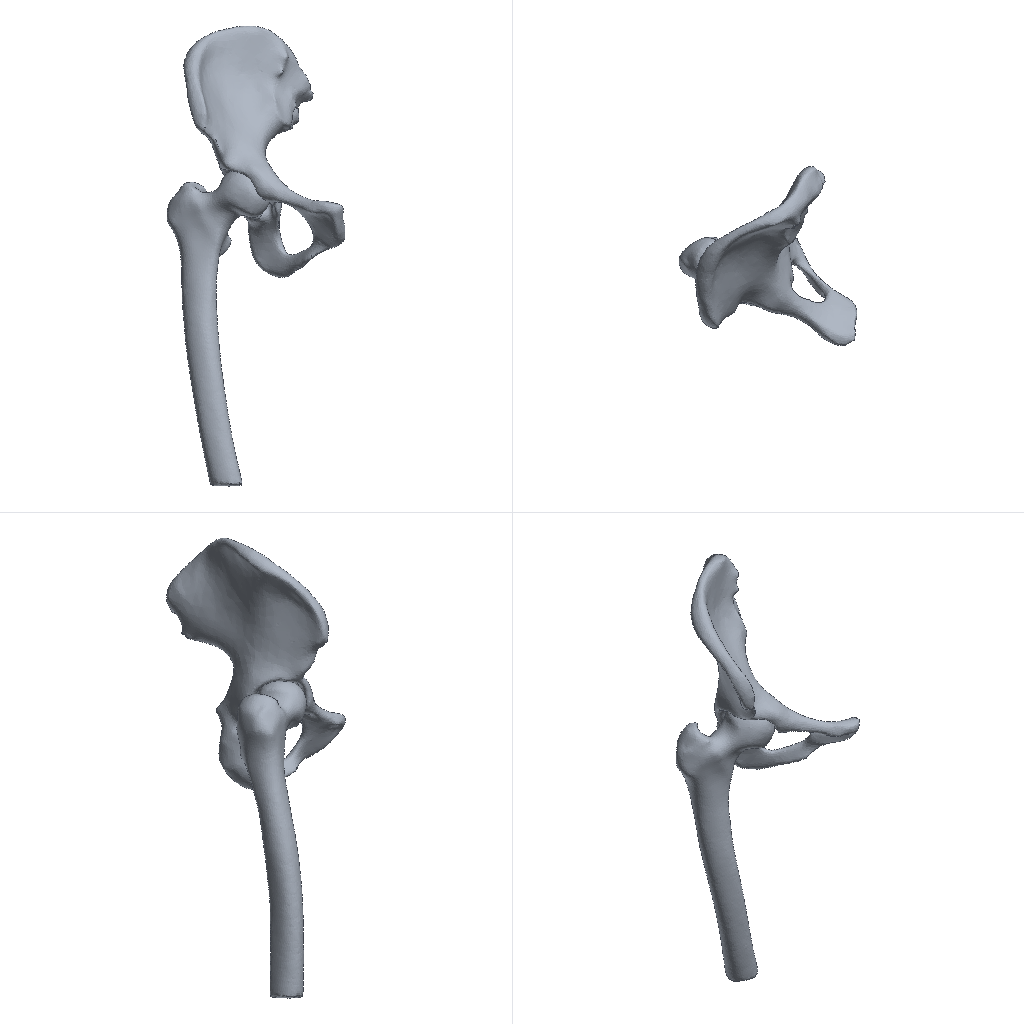Simulation study | abaqus
Set-up summary, first 304 of 512 lines:
category,name,step,type,value,unit,region
solver,abaqus,,Abaqus/CAE 2024
units,unstated,,unstated,E=3.588 density=10 (no match)
analysis,Step-1,,static,time_period=1
mesh,nodes,,,69990
mesh,elements,,,349636
element_type,C3D4,,,349636
material,MAT1,,E,3.588
material,MAT1,,nu,0.3
material,MAT1,,density,10
material,MAT2,,E,3.588
material,MAT2,,nu,0.3
material,MAT2,,density,10
material,MAT3,,E,3.13
material,MAT3,,nu,0.3
material,MAT3,,density,9.163
material,MAT4,,E,25.667
material,MAT4,,nu,0.3
material,MAT4,,density,35.3
material,MAT5,,E,60.925
material,MAT5,,nu,0.3
material,MAT5,,density,61.437
material,MAT6,,E,105.913
material,MAT6,,nu,0.3
material,MAT6,,density,87.574
material,MAT7,,E,159.184
material,MAT7,,nu,0.3
material,MAT7,,density,113.711
material,MAT8,,E,219.822
material,MAT8,,nu,0.3
material,MAT8,,density,139.848
material,MAT9,,E,287.18
material,MAT9,,nu,0.3
material,MAT9,,density,165.985
material,MAT10,,E,360.767
material,MAT10,,nu,0.3
material,MAT10,,density,192.123
material,MAT11,,E,440.194
material,MAT11,,nu,0.3
material,MAT11,,density,218.26
material,MAT12,,E,525.139
material,MAT12,,nu,0.3
material,MAT12,,density,244.397
material,MAT13,,E,615.334
material,MAT13,,nu,0.3
material,MAT13,,density,270.534
material,MAT14,,E,710.549
material,MAT14,,nu,0.3
material,MAT14,,density,296.671
material,MAT15,,E,810.585
material,MAT15,,nu,0.3
material,MAT15,,density,322.808
material,MAT16,,E,915.264
material,MAT16,,nu,0.3
material,MAT16,,density,348.945
material,MAT17,,E,1024.43
material,MAT17,,nu,0.3
material,MAT17,,density,375.083
material,MAT18,,E,1137.94
material,MAT18,,nu,0.3
material,MAT18,,density,401.22
material,MAT19,,E,1255.68
material,MAT19,,nu,0.3
material,MAT19,,density,427.357
material,MAT20,,E,1377.51
material,MAT20,,nu,0.3
material,MAT20,,density,453.494
material,MAT21,,E,1503.35
material,MAT21,,nu,0.3
material,MAT21,,density,479.631
material,MAT22,,E,1633.09
material,MAT22,,nu,0.3
material,MAT22,,density,505.768
material,MAT23,,E,1766.63
material,MAT23,,nu,0.3
material,MAT23,,density,531.905
material,MAT24,,E,1903.91
material,MAT24,,nu,0.3
material,MAT24,,density,558.042
material,MAT25,,E,2044.83
material,MAT25,,nu,0.3
material,MAT25,,density,584.18
material,MAT26,,E,2189.33
material,MAT26,,nu,0.3
material,MAT26,,density,610.317
material,MAT27,,E,2337.34
material,MAT27,,nu,0.3
material,MAT27,,density,636.454
material,MAT28,,E,2488.79
material,MAT28,,nu,0.3
material,MAT28,,density,662.591
material,MAT29,,E,2643.62
material,MAT29,,nu,0.3
material,MAT29,,density,688.728
material,MAT30,,E,2801.78
material,MAT30,,nu,0.3
material,MAT30,,density,714.865
material,MAT31,,E,2963.22
material,MAT31,,nu,0.3
material,MAT31,,density,741.002
material,MAT32,,E,3127.87
material,MAT32,,nu,0.3
material,MAT32,,density,767.139
material,MAT33,,E,3295.7
material,MAT33,,nu,0.3
material,MAT33,,density,793.277
material,MAT34,,E,3466.65
material,MAT34,,nu,0.3
material,MAT34,,density,819.414
material,MAT35,,E,3640.68
material,MAT35,,nu,0.3
material,MAT35,,density,845.551
material,MAT36,,E,3817.76
material,MAT36,,nu,0.3
material,MAT36,,density,871.688
material,MAT37,,E,3997.83
material,MAT37,,nu,0.3
material,MAT37,,density,897.825
material,MAT38,,E,4180.86
material,MAT38,,nu,0.3
material,MAT38,,density,923.962
material,MAT39,,E,4366.81
material,MAT39,,nu,0.3
material,MAT39,,density,950.099
material,MAT40,,E,4555.65
material,MAT40,,nu,0.3
material,MAT40,,density,976.236
material,MAT41,,E,4747.35
material,MAT41,,nu,0.3
material,MAT41,,density,1002.37
material,MAT42,,E,4941.86
material,MAT42,,nu,0.3
material,MAT42,,density,1028.51
material,MAT43,,E,5139.16
material,MAT43,,nu,0.3
material,MAT43,,density,1054.65
material,MAT44,,E,5339.22
material,MAT44,,nu,0.3
material,MAT44,,density,1080.78
material,MAT45,,E,5542.01
material,MAT45,,nu,0.3
material,MAT45,,density,1106.92
material,MAT46,,E,5747.5
material,MAT46,,nu,0.3
material,MAT46,,density,1133.06
material,MAT47,,E,5955.66
material,MAT47,,nu,0.3
material,MAT47,,density,1159.2
material,MAT48,,E,6166.46
material,MAT48,,nu,0.3
material,MAT48,,density,1185.33
material,MAT49,,E,6379.89
material,MAT49,,nu,0.3
material,MAT49,,density,1211.47
material,MAT50,,E,6595.9
material,MAT50,,nu,0.3
material,MAT50,,density,1237.61
material,MAT51,,E,6814.49
material,MAT51,,nu,0.3
material,MAT51,,density,1263.74
material,MAT52,,E,7035.63
material,MAT52,,nu,0.3
material,MAT52,,density,1289.88
material,MAT53,,E,7259.29
material,MAT53,,nu,0.3
material,MAT53,,density,1316.02
material,MAT54,,E,7485.45
material,MAT54,,nu,0.3
material,MAT54,,density,1342.16
material,MAT55,,E,7714.09
material,MAT55,,nu,0.3
material,MAT55,,density,1368.29
material,MAT56,,E,7945.18
material,MAT56,,nu,0.3
material,MAT56,,density,1394.43
material,MAT57,,E,8178.72
material,MAT57,,nu,0.3
material,MAT57,,density,1420.57
material,MAT58,,E,8414.68
material,MAT58,,nu,0.3
material,MAT58,,density,1446.7
material,MAT59,,E,8653.03
material,MAT59,,nu,0.3
material,MAT59,,density,1472.84
material,MAT60,,E,8893.77
material,MAT60,,nu,0.3
material,MAT60,,density,1498.98
material,MAT61,,E,9136.87
material,MAT61,,nu,0.3
material,MAT61,,density,1525.12
material,MAT62,,E,9382.31
material,MAT62,,nu,0.3
material,MAT62,,density,1551.25
material,MAT63,,E,9630.08
material,MAT63,,nu,0.3
material,MAT63,,density,1577.39
material,MAT64,,E,9880.16
material,MAT64,,nu,0.3
material,MAT64,,density,1603.53
material,MAT65,,E,10132.5
material,MAT65,,nu,0.3
material,MAT65,,density,1629.66
material,MAT66,,E,10387.2
material,MAT66,,nu,0.3
material,MAT66,,density,1655.8
material,MAT67,,E,10644.1
material,MAT67,,nu,0.3
material,MAT67,,density,1681.94
material,MAT68,,E,10903.3
material,MAT68,,nu,0.3
material,MAT68,,density,1708.08
material,MAT69,,E,11164.6
material,MAT69,,nu,0.3
material,MAT69,,density,1734.21
material,MAT70,,E,11428.2
material,MAT70,,nu,0.3
material,MAT70,,density,1760.35
material,MAT71,,E,11694
material,MAT71,,nu,0.3
material,MAT71,,density,1786.49
material,MAT72,,E,11962
material,MAT72,,nu,0.3
material,MAT72,,density,1812.62
material,MAT73,,E,12232.2
material,MAT73,,nu,0.3
material,MAT73,,density,1838.76
material,MAT74,,E,12504.5
material,MAT74,,nu,0.3
material,MAT74,,density,1864.9
material,MAT75,,E,12779
material,MAT75,,nu,0.3
material,MAT75,,density,1891.04
material,MAT76,,E,13055.6
material,MAT76,,nu,0.3
material,MAT76,,density,1917.17
material,MAT77,,E,13334.3
material,MAT77,,nu,0.3
material,MAT77,,density,1943.31
material,MAT78,,E,13615.1
material,MAT78,,nu,0.3
material,MAT78,,density,1969.45
material,MAT79,,E,13898.1
material,MAT79,,nu,0.3
material,MAT79,,density,1995.58
material,MAT80,,E,14183.1
material,MAT80,,nu,0.3
material,MAT80,,density,2021.72
material,MAT81,,E,14470.1
material,MAT81,,nu,0.3
material,MAT81,,density,2047.86
material,MAT82,,E,14759.3
material,MAT82,,nu,0.3
material,MAT82,,density,2074
material,MAT83,,E,15050.5
material,MAT83,,nu,0.3
material,MAT83,,density,2100.13
material,MAT84,,E,15343.7
material,MAT84,,nu,0.3
material,MAT84,,density,2126.27
material,MAT85,,E,15638.9
material,MAT85,,nu,0.3
material,MAT85,,density,2152.41
material,MAT86,,E,15936.2
material,MAT86,,nu,0.3
material,MAT86,,density,2178.54
material,MAT87,,E,16235.5
material,MAT87,,nu,0.3
material,MAT87,,density,2204.68
material,MAT88,,E,16536.7
material,MAT88,,nu,0.3
material,MAT88,,density,2230.82
material,MAT89,,E,16840
material,MAT89,,nu,0.3
material,MAT89,,density,2256.96
material,MAT90,,E,17145.2
material,MAT90,,nu,0.3
material,MAT90,,density,2283.09
material,MAT91,,E,17452.3
material,MAT91,,nu,0.3
material,MAT91,,density,2309.23
material,MAT92,,E,17761.5
material,MAT92,,nu,0.3
material,MAT92,,density,2335.37
material,MAT93,,E,18072.5
material,MAT93,,nu,0.3
material,MAT93,,density,2361.5
material,MAT94,,E,18385.6
material,MAT94,,nu,0.3
material,MAT94,,density,2387.64
material,MAT95,,E,18700.5
material,MAT95,,nu,0.3
material,MAT95,,density,2413.78
material,MAT96,,E,19017.3
material,MAT96,,nu,0.3
material,MAT96,,density,2439.92
material,MAT97,,E,19336.1
material,MAT97,,nu,0.3
material,MAT97,,density,2466.05
material,MAT98,,E,19656.7
material,MAT98,,nu,0.3
material,MAT98,,density,2492.19
material,MAT99,,E,19979.3
material,MAT99,,nu,0.3
material,MAT99,,density,2518.33
Abaqus input file, long lists of numbers shortened:
*Heading
** Job name: deck Model name: Model-1
** Generated by: Abaqus/CAE 2024
*Preprint, echo=NO, model=NO, history=NO, contact=NO
**
** PARTS
**
*Part, name=PART-1
*Node
      1,   130.489,   178.725,  -456.04
      2,     128.38,   180.805,  -455.985
** (42545 more lines like these left out)
*Element, type=C3D4
     1, 15021, 15022, 15023, 15024
     2, 15052, 15056, 15061, 15060
** (209817 more lines like these left out)
*Elset, elset=SET1, generate
    1,  5544,     1
*Elset, elset=SET2, generate
  5545,  11304,      1
*Elset, elset=SET3, generate
 11305,  17139,      1
*Elset, elset=SET4, generate
 17140,  21919,      1
*Elset, elset=SET5, generate
 21920,  26644,      1
*Elset, elset=SET6, generate
 26645,  31174,      1
*Elset, elset=SET7, generate
 31175,  35879,      1
*Elset, elset=SET8, generate
 35880,  40947,      1
*Elset, elset=SET9, generate
 40948,  45595,      1
*Elset, elset=SET10, generate
 45596,  50282,      1
*Elset, elset=SET11, generate
 50283,  54802,      1
*Elset, elset=SET12, generate
 54803,  60110,      1
*Elset, elset=SET13, generate
 60111,  64878,      1
*Elset, elset=SET14, generate
 64879,  69715,      1
*Elset, elset=SET15, generate
 69716,  75415,      1
*Elset, elset=SET16, generate
 75416,  80360,      1
*Elset, elset=SET17, generate
 80361,  85668,      1
*Elset, elset=SET18, generate
 85669,  88539,      1
*Elset, elset=SET19, generate
 88540,  92539,      1
*Elset, elset=SET20, generate
 92540,  97409,      1
*Elset, elset=SET21, generate
  97410,  101380,       1
*Elset, elset=SET22, generate
 101381,  104554,       1
*Elset, elset=SET23, generate
 104555,  108745,       1
*Elset, elset=SET24, generate
 108746,  111019,       1
*Elset, elset=SET25, generate
 111020,  114768,       1
*Elset, elset=SET26, generate
 114769,  118305,       1
*Elset, elset=SET27, generate
 118306,  118406,       1
*Elset, elset=SET28, generate
 118407,  120989,       1
*Elset, elset=SET29, generate
 120990,  124573,       1
*Elset, elset=SET30, generate
 124574,  126890,       1
*Elset, elset=SET31, generate
 126891,  130256,       1
*Elset, elset=SET32, generate
 130257,  133204,       1
*Elset, elset=SET33, generate
 133205,  137274,       1
*Elset, elset=SET34, generate
 137275,  139342,       1
*Elset, elset=SET35, generate
 139343,  143097,       1
*Elset, elset=SET36, generate
 143098,  146468,       1
*Elset, elset=SET37, generate
 146469,  150080,       1
*Elset, elset=SET38, generate
 150081,  151210,       1
*Elset, elset=SET39, generate
 151211,  153627,       1
*Elset, elset=SET40, generate
 153628,  155034,       1
*Elset, elset=SET41, generate
 155035,  156868,       1
*Elset, elset=SET42, generate
 156869,  159876,       1
*Elset, elset=SET43, generate
 159877,  162662,       1
*Elset, elset=SET44, generate
 162663,  165367,       1
*Elset, elset=SET45, generate
 165368,  167319,       1
*Elset, elset=SET46, generate
 167320,  167831,       1
*Elset, elset=SET47, generate
 167832,  170587,       1
*Elset, elset=SET48, generate
 170588,  171822,       1
*Elset, elset=SET49, generate
 171823,  174996,       1
*Elset, elset=SET50, generate
 174997,  175669,       1
*Elset, elset=SET51, generate
 175670,  178846,       1
*Elset, elset=SET52, generate
 178847,  179828,       1
*Elset, elset=SET53, generate
 179829,  181183,       1
*Elset, elset=SET54, generate
 181184,  182916,       1
*Elset, elset=SET55, generate
 182917,  183902,       1
*Elset, elset=SET56, generate
 183903,  184076,       1
*Elset, elset=SET57, generate
 184077,  184573,       1
*Elset, elset=SET58, generate
 184574,  186976,       1
*Elset, elset=SET59, generate
 186977,  187814,       1
*Elset, elset=SET60, generate
 187815,  189490,       1
*Elset, elset=SET61, generate
 189491,  189706,       1
*Elset, elset=SET62, generate
 189707,  191900,       1
*Elset, elset=SET63, generate
 191901,  193163,       1
*Elset, elset=SET64, generate
 193164,  195027,       1
*Elset, elset=SET65, generate
 195028,  195725,       1
*Elset, elset=SET66, generate
 195726,  196332,       1
*Elset, elset=SET67, generate
 196333,  197612,       1
*Elset, elset=SET68, generate
 197613,  199159,       1
*Elset, elset=SET69, generate
 199160,  200649,       1
*Elset, elset=SET70, generate
 200650,  201547,       1
*Elset, elset=SET71, generate
 201548,  202707,       1
*Elset, elset=SET72, generate
 202708,  203378,       1
*Elset, elset=SET73, generate
 203379,  203387,       1
*Elset, elset=SET74, generate
 203388,  203647,       1
*Elset, elset=SET75, generate
 203648,  205094,       1
*Elset, elset=SET76, generate
 205095,  205226,       1
*Elset, elset=SET77, generate
 205227,  205780,       1
*Elset, elset=SET78, generate
 205781,  205844,       1
*Elset, elset=SET79, generate
 205845,  206302,       1
*Elset, elset=SET80, generate
 206303,  206457,       1
*Elset, elset=SET81, generate
 206458,  206530,       1
*Elset, elset=SET82, generate
 206531,  206832,       1
*Elset, elset=SET83, generate
 206833,  206849,       1
*Elset, elset=SET84, generate
 206850,  207592,       1
*Elset, elset=SET85, generate
 207593,  207931,       1
*Elset, elset=SET86, generate
 207932,  208213,       1
*Elset, elset=SET87, generate
 208214,  208584,       1
*Elset, elset=SET88, generate
 208585,  208647,       1
*Elset, elset=SET89, generate
 208648,  208986,       1
*Elset, elset=SET90, generate
 208987,  208994,       1
*Elset, elset=SET91, generate
 208995,  209235,       1
*Elset, elset=SET92, generate
 209236,  209268,       1
*Elset, elset=SET93, generate
 209269,  209473,       1
*Elset, elset=SET94, generate
 209474,  209665,       1
*Elset, elset=SET95, generate
 209666,  209783,       1
*Elset, elset=SET96, generate
 209784,  209799,       1
*Elset, elset=SET97, generate
 209800,  209807,       1
*Elset, elset=SET98, generate
 209808,  209811,       1
*Elset, elset=SET99, generate
 209812,  209818,       1
*Elset, elset=SET100
 209819,
** Section: Section-1-SET1
*Solid Section, elset=SET1, material=MAT21
,
** Section: Section-2-SET2
*Solid Section, elset=SET2, material=MAT65
,
** Section: Section-3-SET3
*Solid Section, elset=SET3, material=MAT36
,
** Section: Section-4-SET4
*Solid Section, elset=SET4, material=MAT31
,
** Section: Section-5-SET5
*Solid Section, elset=SET5, material=MAT32
,
** Section: Section-6-SET6
*Solid Section, elset=SET6, material=MAT20
,
** Section: Section-7-SET7
*Solid Section, elset=SET7, material=MAT22
,
** Section: Section-8-SET8
*Solid Section, elset=SET8, material=MAT33
,
** Section: Section-9-SET9
*Solid Section, elset=SET9, material=MAT27
,
** Section: Section-10-SET10
*Solid Section, elset=SET10, material=MAT34
,
** Section: Section-11-SET11
*Solid Section, elset=SET11, material=MAT11
,
** Section: Section-12-SET12
*Solid Section, elset=SET12, material=MAT10
,
** Section: Section-13-SET13
*Solid Section, elset=SET13, material=MAT96
,
** Section: Section-14-SET14
*Solid Section, elset=SET14, material=MAT14
,
** Section: Section-15-SET15
*Solid Section, elset=SET15, material=MAT83
,
** Section: Section-16-SET16
*Solid Section, elset=SET16, material=MAT8
,
** Section: Section-17-SET17
*Solid Section, elset=SET17, material=MAT12
,
** Section: Section-18-SET18
*Solid Section, elset=SET18, material=MAT9
,
** Section: Section-19-SET19
*Solid Section, elset=SET19, material=MAT17
,
** Section: Section-20-SET20
*Solid Section, elset=SET20, material=MAT28
,
** Section: Section-21-SET21
*Solid Section, elset=SET21, material=MAT40
,
** Section: Section-22-SET22
*Solid Section, elset=SET22, material=MAT35
,
** Section: Section-23-SET23
*Solid Section, elset=SET23, material=MAT29
,
** Section: Section-24-SET24
*Solid Section, elset=SET24, material=MAT26
,
** Section: Section-25-SET25
*Solid Section, elset=SET25, material=MAT25
,
** Section: Section-26-SET26
*Solid Section, elset=SET26, material=MAT23
,
** Section: Section-27-SET27
*Solid Section, elset=SET27, material=MAT7
,
** Section: Section-28-SET28
*Solid Section, elset=SET28, material=MAT41
,
** Section: Section-29-SET29
*Solid Section, elset=SET29, material=MAT19
,
** Section: Section-30-SET30
*Solid Section, elset=SET30, material=MAT42
,
** Section: Section-31-SET31
*Solid Section, elset=SET31, material=MAT13
,
** Section: Section-32-SET32
*Solid Section, elset=SET32, material=MAT16
,
** Section: Section-33-SET33
*Solid Section, elset=SET33, material=MAT30
,
** Section: Section-34-SET34
*Solid Section, elset=SET34, material=MAT37
,
** Section: Section-35-SET35
*Solid Section, elset=SET35, material=MAT46
,
** Section: Section-36-SET36
*Solid Section, elset=SET36, material=MAT15
,
** Section: Section-37-SET37
*Solid Section, elset=SET37, material=MAT91
,
** Section: Section-38-SET38
*Solid Section, elset=SET38, material=MAT6
,
** Section: Section-39-SET39
*Solid Section, elset=SET39, material=MAT4
,
** Section: Section-40-SET40
*Solid Section, elset=SET40, material=MAT2
,
** Section: Section-41-SET41
*Solid Section, elset=SET41, material=MAT3
,
** Section: Section-42-SET42
*Solid Section, elset=SET42, material=MAT5
,
** Section: Section-43-SET43
*Solid Section, elset=SET43, material=MAT39
,
** Section: Section-44-SET44
*Solid Section, elset=SET44, material=MAT90
,
** Section: Section-45-SET45
*Solid Section, elset=SET45, material=MAT38
,
** Section: Section-46-SET46
*Solid Section, elset=SET46, material=MAT80
,
** Section: Section-47-SET47
*Solid Section, elset=SET47, material=MAT52
,
** Section: Section-48-SET48
*Solid Section, elset=SET48, material=MAT86
,
** Section: Section-49-SET49
*Solid Section, elset=SET49, material=MAT24
,
** Section: Section-50-SET50
*Solid Section, elset=SET50, material=MAT43
,
** Section: Section-51-SET51
*Solid Section, elset=SET51, material=MAT76
,
** Section: Section-52-SET52
*Solid Section, elset=SET52, material=MAT95
,
** Section: Section-53-SET53
*Solid Section, elset=SET53, material=MAT93
,
** Section: Section-54-SET54
*Solid Section, elset=SET54, material=MAT89
,
** Section: Section-55-SET55
*Solid Section, elset=SET55, material=MAT45
,
** Section: Section-56-SET56
*Solid Section, elset=SET56, material=MAT44
,
** Section: Section-57-SET57
*Solid Section, elset=SET57, material=MAT18
,
** Section: Section-58-SET58
*Solid Section, elset=SET58, material=MAT54
,
** Section: Section-59-SET59
*Solid Section, elset=SET59, material=MAT77
,
** Section: Section-60-SET60
*Solid Section, elset=SET60, material=MAT71
,
** Section: Section-61-SET61
*Solid Section, elset=SET61, material=MAT55
,
** Section: Section-62-SET62
*Solid Section, elset=SET62, material=MAT73
,
** Section: Section-63-SET63
*Solid Section, elset=SET63, material=MAT47
,
** Section: Section-64-SET64
*Solid Section, elset=SET64, material=MAT67
,
** Section: Section-65-SET65
*Solid Section, elset=SET65, material=MAT81
,
** Section: Section-66-SET66
*Solid Section, elset=SET66, material=MAT59
,
** Section: Section-67-SET67
*Solid Section, elset=SET67, material=MAT78
,
** Section: Section-68-SET68
*Solid Section, elset=SET68, material=MAT49
,
** Section: Section-69-SET69
*Solid Section, elset=SET69, material=MAT51
,
** Section: Section-70-SET70
*Solid Section, elset=SET70, material=MAT87
,
** Section: Section-71-SET71
*Solid Section, elset=SET71, material=MAT74
,
** Section: Section-72-SET72
*Solid Section, elset=SET72, material=MAT88
,
** Section: Section-73-SET73
*Solid Section, elset=SET73, material=MAT62
,
** Section: Section-74-SET74
*Solid Section, elset=SET74, material=MAT58
,
** Section: Section-75-SET75
*Solid Section, elset=SET75, material=MAT53
,
** Section: Section-76-SET76
*Solid Section, elset=SET76, material=MAT82
,
** Section: Section-77-SET77
*Solid Section, elset=SET77, material=MAT92
,
** Section: Section-78-SET78
*Solid Section, elset=SET78, material=MAT57
,
** Section: Section-79-SET79
*Solid Section, elset=SET79, material=MAT68
,
** Section: Section-80-SET80
*Solid Section, elset=SET80, material=MAT97
,
** Section: Section-81-SET81
*Solid Section, elset=SET81, material=MAT60
,
** Section: Section-82-SET82
*Solid Section, elset=SET82, material=MAT1
,
** Section: Section-83-SET83
*Solid Section, elset=SET83, material=MAT61
,
** Section: Section-84-SET84
*Solid Section, elset=SET84, material=MAT50
,
** Section: Section-85-SET85
*Solid Section, elset=SET85, material=MAT66
,
** Section: Section-86-SET86
*Solid Section, elset=SET86, material=MAT84
,
** Section: Section-87-SET87
*Solid Section, elset=SET87, material=MAT63
,
** Section: Section-88-SET88
*Solid Section, elset=SET88, material=MAT85
,
** Section: Section-89-SET89
*Solid Section, elset=SET89, material=MAT64
,
** Section: Section-90-SET90
*Solid Section, elset=SET90, material=MAT94
,
** Section: Section-91-SET91
*Solid Section, elset=SET91, material=MAT56
,
** Section: Section-92-SET92
*Solid Section, elset=SET92, material=MAT72
,
** Section: Section-93-SET93
*Solid Section, elset=SET93, material=MAT75
,
** Section: Section-94-SET94
*Solid Section, elset=SET94, material=MAT48
,
** Section: Section-95-SET95
*Solid Section, elset=SET95, material=MAT79
,
** Section: Section-96-SET96
*Solid Section, elset=SET96, material=MAT69
,
** Section: Section-97-SET97
*Solid Section, elset=SET97, material=MAT70
,
** Section: Section-98-SET98
*Solid Section, elset=SET98, material=MAT99
,
** Section: Section-99-SET99
*Solid Section, elset=SET99, material=MAT98
,
** Section: Section-100-SET100
*Solid Section, elset=SET100, material=MAT100
,
*End Part
**
*Part, name=PART-2
*Node
      1,   84.384,   152.255,  -622.89
      2,    85.776,   150.316,  -622.89
** (27441 more lines like these left out)
*Element, type=C3D4
     1,  8146,  8147,  8148,  8149
     2,  8238,  8239,  8240,  8241
** (139815 more lines like these left out)
*Elset, elset=SET1, generate
    1,  2335,     1
*Elset, elset=SET2, generate
 2336,  3097,     1
*Elset, elset=SET3, generate
 3098,  4149,     1
*Elset, elset=SET4, generate
 4150,  5553,     1
*Elset, elset=SET5, generate
 5554,  6887,     1
*Elset, elset=SET6, generate
 6888,  9154,     1
*Elset, elset=SET7, generate
  9155,  11513,      1
*Elset, elset=SET8, generate
 11514,  12802,      1
*Elset, elset=SET9, generate
 12803,  14643,      1
*Elset, elset=SET10, generate
 14644,  15767,      1
*Elset, elset=SET11, generate
 15768,  18886,      1
*Elset, elset=SET12, generate
 18887,  22084,      1
*Elset, elset=SET13, generate
 22085,  22681,      1
*Elset, elset=SET14, generate
 22682,  25288,      1
*Elset, elset=SET15, generate
 25289,  26507,      1
*Elset, elset=SET16, generate
 26508,  29349,      1
*Elset, elset=SET17, generate
 29350,  32184,      1
*Elset, elset=SET18, generate
 32185,  35205,      1
*Elset, elset=SET19, generate
 35206,  37703,      1
*Elset, elset=SET20, generate
 37704,  39334,      1
*Elset, elset=SET21, generate
 39335,  40183,      1
*Elset, elset=SET22, generate
 40184,  41305,      1
*Elset, elset=SET23, generate
 41306,  42847,      1
*Elset, elset=SET24, generate
 42848,  44901,      1
*Elset, elset=SET25, generate
 44902,  47087,      1
*Elset, elset=SET26, generate
 47088,  49240,      1
*Elset, elset=SET27, generate
 49241,  51990,      1
*Elset, elset=SET28, generate
 51991,  52916,      1
*Elset, elset=SET29, generate
 52917,  55309,      1
*Elset, elset=SET30, generate
 55310,  56192,      1
*Elset, elset=SET31, generate
 56193,  58885,      1
*Elset, elset=SET32, generate
 58886,  61412,      1
*Elset, elset=SET33, generate
 61413,  62931,      1
*Elset, elset=SET34, generate
 62932,  64000,      1
*Elset, elset=SET35, generate
 64001,  64801,      1
*Elset, elset=SET36, generate
 64802,  67370,      1
*Elset, elset=SET37, generate
 67371,  70024,      1
*Elset, elset=SET38, generate
 70025,  72673,      1
*Elset, elset=SET39, generate
 72674,  74527,      1
*Elset, elset=SET40, generate
 74528,  74897,      1
*Elset, elset=SET41, generate
 74898,  75883,      1
*Elset, elset=SET42, generate
 75884,  78340,      1
*Elset, elset=SET43, generate
 78341,  79304,      1
*Elset, elset=SET44, generate
 79305,  81908,      1
*Elset, elset=SET45, generate
 81909,  82930,      1
*Elset, elset=SET46, generate
 82931,  83998,      1
*Elset, elset=SET47, generate
 83999,  84855,      1
*Elset, elset=SET48, generate
 84856,  86755,      1
*Elset, elset=SET49, generate
 86756,  89023,      1
*Elset, elset=SET50, generate
 89024,  89864,      1
*Elset, elset=SET51, generate
 89865,  90735,      1
*Elset, elset=SET52, generate
 90736,  91954,      1
*Elset, elset=SET53, generate
 91955,  94110,      1
*Elset, elset=SET54, generate
 94111,  96693,      1
*Elset, elset=SET55, generate
 96694,  97444,      1
*Elset, elset=SET56, generate
 97445,  98232,      1
*Elset, elset=SET57, generate
  98233,  100679,       1
*Elset, elset=SET58, generate
 100680,  101512,       1
*Elset, elset=SET59, generate
 101513,  102438,       1
*Elset, elset=SET60, generate
 102439,  103233,       1
*Elset, elset=SET61, generate
 103234,  104059,       1
*Elset, elset=SET62, generate
 104060,  104899,       1
*Elset, elset=SET63, generate
 104900,  105728,       1
*Elset, elset=SET64, generate
 105729,  106519,       1
*Elset, elset=SET65, generate
 106520,  107514,       1
*Elset, elset=SET66, generate
 107515,  108291,       1
*Elset, elset=SET67, generate
 108292,  109246,       1
*Elset, elset=SET68, generate
 109247,  110107,       1
*Elset, elset=SET69, generate
 110108,  110992,       1
*Elset, elset=SET70, generate
 110993,  113025,       1
*Elset, elset=SET71, generate
 113026,  113898,       1
*Elset, elset=SET72, generate
 113899,  116284,       1
*Elset, elset=SET73, generate
 116285,  117031,       1
*Elset, elset=SET74, generate
 117032,  117782,       1
*Elset, elset=SET75, generate
 117783,  118617,       1
*Elset, elset=SET76, generate
 118618,  119815,       1
*Elset, elset=SET77, generate
 119816,  122531,       1
*Elset, elset=SET78, generate
 122532,  123263,       1
*Elset, elset=SET79, generate
 123264,  124071,       1
*Elset, elset=SET80, generate
 124072,  124307,       1
*Elset, elset=SET81, generate
 124308,  125023,       1
*Elset, elset=SET82, generate
 125024,  125089,       1
*Elset, elset=SET83, generate
 125090,  125884,       1
*Elset, elset=SET84, generate
 125885,  126748,       1
*Elset, elset=SET85, generate
 126749,  127475,       1
*Elset, elset=SET86, generate
 127476,  128877,       1
*Elset, elset=SET87, generate
 128878,  129637,       1
*Elset, elset=SET88, generate
 129638,  131173,       1
*Elset, elset=SET89, generate
 131174,  131920,       1
*Elset, elset=SET90, generate
 131921,  133702,       1
*Elset, elset=SET91, generate
 133703,  134533,       1
*Elset, elset=SET92, generate
 134534,  135387,       1
*Elset, elset=SET93, generate
 135388,  136238,       1
*Elset, elset=SET94, generate
 136239,  137053,       1
*Elset, elset=SET95, generate
 137054,  138015,       1
*Elset, elset=SET96, generate
 138016,  138823,       1
*Elset, elset=SET97, generate
 138824,  139639,       1
*Elset, elset=SET98, generate
 139640,  139707,       1
*Elset, elset=SET99, generate
 139708,  139797,       1
*Elset, elset=SET100, generate
 139798,  139817,       1
** Section: Section-1-SET1
*Solid Section, elset=SET1, material=MAT21
,
** Section: Section-2-SET2
*Solid Section, elset=SET2, material=MAT65
,
** Section: Section-3-SET3
*Solid Section, elset=SET3, material=MAT36
,
** Section: Section-4-SET4
*Solid Section, elset=SET4, material=MAT31
,
** Section: Section-5-SET5
*Solid Section, elset=SET5, material=MAT32
,
** Section: Section-6-SET6
*Solid Section, elset=SET6, material=MAT20
,
** Section: Section-7-SET7
*Solid Section, elset=SET7, material=MAT22
,
** Section: Section-8-SET8
*Solid Section, elset=SET8, material=MAT33
,
** Section: Section-9-SET9
*Solid Section, elset=SET9, material=MAT27
,
** Section: Section-10-SET10
*Solid Section, elset=SET10, material=MAT34
,
** Section: Section-11-SET11
*Solid Section, elset=SET11, material=MAT11
,
** Section: Section-12-SET12
*Solid Section, elset=SET12, material=MAT10
,
** Section: Section-13-SET13
*Solid Section, elset=SET13, material=MAT96
,
** Section: Section-14-SET14
*Solid Section, elset=SET14, material=MAT14
,
** Section: Section-15-SET15
*Solid Section, elset=SET15, material=MAT83
,
** Section: Section-16-SET16
*Solid Section, elset=SET16, material=MAT8
,
** Section: Section-17-SET17
*Solid Section, elset=SET17, material=MAT12
,
** Section: Section-18-SET18
*Solid Section, elset=SET18, material=MAT9
,
** Section: Section-19-SET19
*Solid Section, elset=SET19, material=MAT17
,
** Section: Section-20-SET20
*Solid Section, elset=SET20, material=MAT28
,
** Section: Section-21-SET21
*Solid Section, elset=SET21, material=MAT40
,
** Section: Section-22-SET22
*Solid Section, elset=SET22, material=MAT35
,
** Section: Section-23-SET23
*Solid Section, elset=SET23, material=MAT29
,
** Section: Section-24-SET24
*Solid Section, elset=SET24, material=MAT26
,
** Section: Section-25-SET25
*Solid Section, elset=SET25, material=MAT25
,
** Section: Section-26-SET26
*Solid Section, elset=SET26, material=MAT23
,
** Section: Section-27-SET27
*Solid Section, elset=SET27, material=MAT7
,
** Section: Section-28-SET28
*Solid Section, elset=SET28, material=MAT41
,
** Section: Section-29-SET29
*Solid Section, elset=SET29, material=MAT19
,
** Section: Section-30-SET30
*Solid Section, elset=SET30, material=MAT42
,
** Section: Section-31-SET31
*Solid Section, elset=SET31, material=MAT13
,
** Section: Section-32-SET32
*Solid Section, elset=SET32, material=MAT16
,
** Section: Section-33-SET33
*Solid Section, elset=SET33, material=MAT30
,
** Section: Section-34-SET34
*Solid Section, elset=SET34, material=MAT37
,
** Section: Section-35-SET35
*Solid Section, elset=SET35, material=MAT46
,
** Section: Section-36-SET36
*Solid Section, elset=SET36, material=MAT15
,
** Section: Section-37-SET37
*Solid Section, elset=SET37, material=MAT91
,
** Section: Section-38-SET38
*Solid Section, elset=SET38, material=MAT6
,
** Section: Section-39-SET39
*Solid Section, elset=SET39, material=MAT4
,
** Section: Section-40-SET40
*Solid Section, elset=SET40, material=MAT2
,
** Section: Section-41-SET41
*Solid Section, elset=SET41, material=MAT3
,
** Section: Section-42-SET42
*Solid Section, elset=SET42, material=MAT5
,
** Section: Section-43-SET43
*Solid Section, elset=SET43, material=MAT39
,
** Section: Section-44-SET44
*Solid Section, elset=SET44, material=MAT90
,
** Section: Section-45-SET45
*Solid Section, elset=SET45, material=MAT38
,
** Section: Section-46-SET46
*Solid Section, elset=SET46, material=MAT80
,
** Section: Section-47-SET47
*Solid Section, elset=SET47, material=MAT52
,
** Section: Section-48-SET48
*Solid Section, elset=SET48, material=MAT86
,
** Section: Section-49-SET49
*Solid Section, elset=SET49, material=MAT24
,
** Section: Section-50-SET50
*Solid Section, elset=SET50, material=MAT43
,
** Section: Section-51-SET51
*Solid Section, elset=SET51, material=MAT76
,
** Section: Section-52-SET52
*Solid Section, elset=SET52, material=MAT95
,
** Section: Section-53-SET53
*Solid Section, elset=SET53, material=MAT93
,
** Section: Section-54-SET54
*Solid Section, elset=SET54, material=MAT89
,
** Section: Section-55-SET55
*Solid Section, elset=SET55, material=MAT45
,
** Section: Section-56-SET56
*Solid Section, elset=SET56, material=MAT44
,
** Section: Section-57-SET57
*Solid Section, elset=SET57, material=MAT18
,
** Section: Section-58-SET58
*Solid Section, elset=SET58, material=MAT54
,
** Section: Section-59-SET59
*Solid Section, elset=SET59, material=MAT77
,
** Section: Section-60-SET60
*Solid Section, elset=SET60, material=MAT71
,
** Section: Section-61-SET61
*Solid Section, elset=SET61, material=MAT55
,
** Section: Section-62-SET62
*Solid Section, elset=SET62, material=MAT73
,
** Section: Section-63-SET63
*Solid Section, elset=SET63, material=MAT47
,
** Section: Section-64-SET64
*Solid Section, elset=SET64, material=MAT67
,
** Section: Section-65-SET65
*Solid Section, elset=SET65, material=MAT81
,
** Section: Section-66-SET66
*Solid Section, elset=SET66, material=MAT59
,
** Section: Section-67-SET67
*Solid Section, elset=SET67, material=MAT78
,
** Section: Section-68-SET68
*Solid Section, elset=SET68, material=MAT49
,
** Section: Section-69-SET69
*Solid Section, elset=SET69, material=MAT51
,
** Section: Section-70-SET70
*Solid Section, elset=SET70, material=MAT87
,
** Section: Section-71-SET71
*Solid Section, elset=SET71, material=MAT74
,
** Section: Section-72-SET72
*Solid Section, elset=SET72, material=MAT88
,
** Section: Section-73-SET73
*Solid Section, elset=SET73, material=MAT62
,
** Section: Section-74-SET74
*Solid Section, elset=SET74, material=MAT58
,
** Section: Section-75-SET75
*Solid Section, elset=SET75, material=MAT53
,
** Section: Section-76-SET76
*Solid Section, elset=SET76, material=MAT82
,
** Section: Section-77-SET77
*Solid Section, elset=SET77, material=MAT92
,
** Section: Section-78-SET78
*Solid Section, elset=SET78, material=MAT57
,
** Section: Section-79-SET79
*Solid Section, elset=SET79, material=MAT68
,
** Section: Section-80-SET80
*Solid Section, elset=SET80, material=MAT97
,
** Section: Section-81-SET81
*Solid Section, elset=SET81, material=MAT60
,
** Section: Section-82-SET82
*Solid Section, elset=SET82, material=MAT1
,
** Section: Section-83-SET83
*Solid Section, elset=SET83, material=MAT61
,
** Section: Section-84-SET84
*Solid Section, elset=SET84, material=MAT50
,
** Section: Section-85-SET85
*Solid Section, elset=SET85, material=MAT66
,
** Section: Section-86-SET86
*Solid Section, elset=SET86, material=MAT84
,
** Section: Section-87-SET87
*Solid Section, elset=SET87, material=MAT63
,
** Section: Section-88-SET88
*Solid Section, elset=SET88, material=MAT85
,
** Section: Section-89-SET89
*Solid Section, elset=SET89, material=MAT64
,
** Section: Section-90-SET90
*Solid Section, elset=SET90, material=MAT94
,
** Section: Section-91-SET91
*Solid Section, elset=SET91, material=MAT56
,
** Section: Section-92-SET92
*Solid Section, elset=SET92, material=MAT72
,
** Section: Section-93-SET93
*Solid Section, elset=SET93, material=MAT75
,
** Section: Section-94-SET94
*Solid Section, elset=SET94, material=MAT48
,
** Section: Section-95-SET95
*Solid Section, elset=SET95, material=MAT79
,
** Section: Section-96-SET96
*Solid Section, elset=SET96, material=MAT69
,
** Section: Section-97-SET97
*Solid Section, elset=SET97, material=MAT70
,
** Section: Section-98-SET98
*Solid Section, elset=SET98, material=MAT99
,
** Section: Section-99-SET99
*Solid Section, elset=SET99, material=MAT98
,
** Section: Section-100-SET100
*Solid Section, elset=SET100, material=MAT100
,
*End Part
**
**
** ASSEMBLY
**
*Assembly, name=Assembly
**
*Instance, name=PART-1-1, part=PART-1
*End Instance
**
*Instance, name=PART-1-2, part=PART-2
    2.776,     0.3741,     0.7858
*End Instance
**
*Nset, nset=Set-1, instance=PART-1-1
  7620,  7674,  7715,  7741,  7770,  7792,  7867,  7888,  7893,  7927,  7937,  7944,  7952,  8014,  8022,  8043
  8092,  8129,  8178,  8194,  8235,  8288,  8298,  8300,  8325,  8344,  8351,  8407,  8421,  8422,  8435,  8451
** (3 more lines like these left out)
*Nset, nset=Set-2, instance=PART-1-2
     1,     2,     3,     4,     5,     6,     7,     8,     9,    10,    11,    12,    13,    14,    15,    16
    17,    18,    19,    20,    21,    22,    23,    24,    25,    26,    27,    28,    29,    30,    31,    32
** (7 more lines like these left out)
*Nset, nset=Set-3, instance=PART-1-2
 12125,
*Nset, nset=Set-3, instance=PART-1-1
  6389,  6474,  6679,  6685,  6759,  6789,  6887,  6934,  7009, 15059
*Nset, nset=Set-4, instance=PART-1-1
 5813, 6026, 6059, 6334, 6478, 6628, 6734, 6740, 6782, 6928
*Nset, nset=Set-5, instance=PART-1-1
 6272,
*Nset, nset=Set-6, instance=PART-1-1
  1902,  1997,  2004,  2108,  2122,  2135,  2144,  2205,  2224,  2248,  2284,  2325,  2348,  2354,  2402,  2411
  2523,  2530,  2538,  2591,  2680,  2695,  2709,  2729,  2790,  2817,  2899,  2902,  2946,  3005,  3052,  3076
** (1 more lines like these left out)
*Nset, nset=Set-7, instance=PART-1-1
  5653,  5803,  6179,  6261,  6389,  6535,  6628,  6789,  6874, 39732
*Nset, nset=Set-8, instance=PART-1-1
 1854, 1902, 1942, 1997, 2065, 2108, 2191, 2292, 2325, 2346, 2354, 2530, 2538, 2695, 2731, 2870
 2946, 3005, 3264
*Nset, nset=Set-9, instance=PART-1-1
  1956,  2065,  2198,  2227,  2325,  2348,  2411,  2631,  2680,  2709,  2790,  3052,  3076,  3096,  3112, 21492
 26978,
*Nset, nset=Set-10, instance=PART-1-1
  1794,  1854,  1902,  1922,  1938,  1953,  1956,  1997,  2004,  2033,  2034,  2065,  2082,  2113,  2114,  2122
  2144,  2171,  2198,  2205,  2224,  2226,  2237,  2248,  2251,  2295,  2322,  2325,  2341,  2348,  2402,  2406
** (2 more lines like these left out)
*Nset, nset=Set-11, instance=PART-1-1
 5853, 5984, 6161, 6472, 6555, 6570, 6600, 6611, 6789, 6821
*Elset, elset=_Surf-KX_S1, internal, instance=PART-1-2
   319,  1799,  1814,  2264,  3419,  4071,  6614,  6626,  8007, 10196, 11502, 12148, 12168, 13440, 14962, 15615
 15747, 23431, 24255, 35714, 37507, 39177, 39233, 40429, 40756, 41117, 41411, 43686, 46485, 46639, 47036, 48860
** (1 more lines like these left out)
*Elset, elset=_Surf-KX_S2, internal, instance=PART-1-2
   490,  4526,  5754,  5870,  6123,  7945,  9746, 10313, 10323, 11687, 11834, 11971, 13543, 15384, 38203, 38301
 40534, 41658, 43320, 43627, 43800, 45551, 45629, 45710, 46046, 48033, 48039, 53427, 53451, 54225, 55839, 56985
** (2 more lines like these left out)
*Elset, elset=_Surf-KX_S3, internal, instance=PART-1-2
   264,   275,   282,   354,   412,   477,   478,   491,   499,   505,   510,   512,   536,   543,   548,   558
   607,   612,   616,   622,   656,   678,   681,   708,   712,   717,   719,   722,   726,   790,   792,   793
** (103 more lines like these left out)
*Elset, elset=_Surf-KX_S4, internal, instance=PART-1-2
   525,   821,  1104,  1395,  2134,  3349,  3931,  4417,  4725,  4795,  5124,  5231,  5576,  6015,  6099,  7336
  7943,  7966,  8018,  8132,  8545,  8652,  9422,  9900, 11774, 11948, 13102, 13401, 14214, 15038, 15511, 18037
** (4 more lines like these left out)
*Surface, type=ELEMENT, name=Surf-KX
_Surf-KX_S1, S1
_Surf-KX_S2, S2
_Surf-KX_S4, S4
_Surf-KX_S3, S3
*Elset, elset=_Surf-KX1_S1, internal, instance=PART-1-1
   3498,   4016,   8916,  17803,  24023,  25626,  27944,  39381,  39875,  42713,  44880,  45256,  49415,  50193,  50924,  53313
  60717,  69150,  73100,  79188,  79406,  86916,  87584,  91412,  97834,  97888, 107096, 111596, 112109, 113048, 114097, 114282
** (1 more lines like these left out)
*Elset, elset=_Surf-KX1_S2, internal, instance=PART-1-1
  14051,  18325,  18339,  20858,  22168,  22515,  22622,  23831,  28055,  28058,  28480,  30637,  33129,  37087,  41865,  41868
  41922,  46444,  46881,  46948,  51564,  51782,  56461,  60188,  60880,  62041,  62841,  65985,  66009,  67152,  72210,  72668
** (2 more lines like these left out)
*Elset, elset=_Surf-KX1_S3, internal, instance=PART-1-1
    744,   1416,   1465,   1467,   1483,   2245,   2246,   2384,   2479,   2492,   2503,   2518,   2521,   2617,   2622,   2624
   2633,   2636,   2811,   2815,   2819,   2993,   2994,   3011,   3016,   3029,   3589,   3647,   6466,   7162,   7252,   7264
** (106 more lines like these left out)
*Elset, elset=_Surf-KX1_S4, internal, instance=PART-1-1
  12036,  12953,  15528,  15994,  17818,  19982,  23252,  24889,  25422,  27924,  28187,  30014,  31931,  32116,  32183,  34573
  38176,  39547,  40832,  43722,  44353,  44420,  49132,  52203,  52219,  53643,  55642,  60973,  62525,  63016,  63744,  63844
** (3 more lines like these left out)
*Surface, type=ELEMENT, name=Surf-KX1
_Surf-KX1_S1, S1
_Surf-KX1_S2, S2
_Surf-KX1_S4, S4
_Surf-KX1_S3, S3
*Nset, nset="_T-Datum csys-3", internal
Set-10,
*Transform, nset="_T-Datum csys-3"
0.02051, 0.008337, 0.9998, 0.02085, -0.9998, 0.007909
*Nset, nset="_T-Datum csys-4", internal
Set-11,
*Transform, nset="_T-Datum csys-4"
-0.2528, 0.008127, -0.9675, -0.7991, -0.5655, 0.2041
*End Assembly
**
** MATERIALS
**
*Material, name=MAT1
*Density
10.,
*Elastic
 3.588, 0.3
*Material, name=MAT2
*Density
10.,
*Elastic
 3.588, 0.3
*Material, name=MAT3
*Density
 9.163,
*Elastic
 3.13, 0.3
*Material, name=MAT4
*Density
 35.3,
*Elastic
 25.667, 0.3
*Material, name=MAT5
*Density
 61.437,
*Elastic
 60.925, 0.3
*Material, name=MAT6
*Density
 87.574,
*Elastic
 105.913, 0.3
*Material, name=MAT7
*Density
 113.711,
*Elastic
 159.184, 0.3
*Material, name=MAT8
*Density
 139.848,
*Elastic
 219.822, 0.3
*Material, name=MAT9
*Density
 165.985,
*Elastic
 287.18, 0.3
*Material, name=MAT10
*Density
 192.123,
*Elastic
 360.767, 0.3
*Material, name=MAT11
*Density
 218.26,
*Elastic
 440.194, 0.3
*Material, name=MAT12
*Density
 244.397,
*Elastic
 525.139, 0.3
*Material, name=MAT13
*Density
 270.534,
*Elastic
 615.334, 0.3
*Material, name=MAT14
*Density
 296.671,
*Elastic
 710.549, 0.3
*Material, name=MAT15
*Density
 322.808,
*Elastic
 810.585, 0.3
*Material, name=MAT16
*Density
 348.945,
*Elastic
 915.264, 0.3
*Material, name=MAT17
*Density
 375.083,
*Elastic
 1024.43, 0.3
*Material, name=MAT18
*Density
 401.22,
*Elastic
 1137.94, 0.3
*Material, name=MAT19
*Density
 427.357,
*Elastic
 1255.68, 0.3
*Material, name=MAT20
*Density
 453.494,
*Elastic
 1377.51, 0.3
*Material, name=MAT21
*Density
 479.631,
*Elastic
 1503.35, 0.3
*Material, name=MAT22
*Density
 505.768,
*Elastic
 1633.09, 0.3
*Material, name=MAT23
*Density
 531.905,
*Elastic
 1766.63, 0.3
*Material, name=MAT24
*Density
 558.042,
*Elastic
 1903.91, 0.3
*Material, name=MAT25
*Density
 584.18,
*Elastic
 2044.83, 0.3
*Material, name=MAT26
*Density
 610.317,
*Elastic
 2189.33, 0.3
*Material, name=MAT27
*Density
 636.454,
*Elastic
 2337.34, 0.3
*Material, name=MAT28
*Density
 662.591,
*Elastic
 2488.79, 0.3
*Material, name=MAT29
*Density
 688.728,
*Elastic
 2643.62, 0.3
*Material, name=MAT30
*Density
 714.865,
*Elastic
 2801.78, 0.3
*Material, name=MAT31
*Density
 741.002,
*Elastic
 2963.22, 0.3
*Material, name=MAT32
*Density
 767.139,
*Elastic
 3127.87, 0.3
*Material, name=MAT33
*Density
 793.277,
*Elastic
 3295.7, 0.3
*Material, name=MAT34
*Density
 819.414,
*Elastic
 3466.65, 0.3
*Material, name=MAT35
*Density
 845.551,
*Elastic
 3640.68, 0.3
*Material, name=MAT36
*Density
 871.688,
*Elastic
 3817.76, 0.3
*Material, name=MAT37
*Density
 897.825,
*Elastic
 3997.83, 0.3
*Material, name=MAT38
*Density
 923.962,
*Elastic
 4180.86, 0.3
*Material, name=MAT39
*Density
 950.099,
*Elastic
 4366.81, 0.3
*Material, name=MAT40
*Density
 976.236,
*Elastic
 4555.65, 0.3
*Material, name=MAT41
*Density
 1002.37,
*Elastic
 4747.35, 0.3
*Material, name=MAT42
*Density
 1028.51,
*Elastic
 4941.86, 0.3
*Material, name=MAT43
*Density
 1054.65,
*Elastic
 5139.16, 0.3
*Material, name=MAT44
*Density
 1080.78,
*Elastic
 5339.22, 0.3
*Material, name=MAT45
*Density
 1106.92,
*Elastic
 5542.01, 0.3
*Material, name=MAT46
*Density
 1133.06,
*Elastic
 5747.5, 0.3
*Material, name=MAT47
*Density
 1159.2,
*Elastic
 5955.66, 0.3
*Material, name=MAT48
*Density
 1185.33,
*Elastic
 6166.46, 0.3
*Material, name=MAT49
*Density
 1211.47,
*Elastic
 6379.89, 0.3
*Material, name=MAT50
*Density
 1237.61,
*Elastic
 6595.9, 0.3
*Material, name=MAT51
*Density
 1263.74,
*Elastic
 6814.49, 0.3
*Material, name=MAT52
*Density
 1289.88,
*Elastic
 7035.63, 0.3
*Material, name=MAT53
*Density
 1316.02,
*Elastic
 7259.29, 0.3
*Material, name=MAT54
*Density
 1342.16,
*Elastic
 7485.45, 0.3
*Material, name=MAT55
*Density
 1368.29,
*Elastic
 7714.09, 0.3
*Material, name=MAT56
*Density
 1394.43,
*Elastic
 7945.18, 0.3
*Material, name=MAT57
*Density
 1420.57,
*Elastic
 8178.72, 0.3
*Material, name=MAT58
*Density
 1446.7,
*Elastic
 8414.68, 0.3
*Material, name=MAT59
*Density
 1472.84,
*Elastic
 8653.03, 0.3
*Material, name=MAT60
*Density
 1498.98,
*Elastic
 8893.77, 0.3
*Material, name=MAT61
*Density
 1525.12,
*Elastic
 9136.87, 0.3
*Material, name=MAT62
*Density
 1551.25,
*Elastic
 9382.31, 0.3
*Material, name=MAT63
*Density
 1577.39,
*Elastic
 9630.08, 0.3
*Material, name=MAT64
*Density
 1603.53,
*Elastic
 9880.16, 0.3
*Material, name=MAT65
*Density
 1629.66,
*Elastic
 10132.5, 0.3
*Material, name=MAT66
*Density
 1655.8,
*Elastic
 10387.2, 0.3
*Material, name=MAT67
*Density
 1681.94,
*Elastic
 10644.1, 0.3
*Material, name=MAT68
*Density
 1708.08,
*Elastic
 10903.3, 0.3
*Material, name=MAT69
*Density
 1734.21,
*Elastic
 11164.6, 0.3
*Material, name=MAT70
*Density
 1760.35,
*Elastic
 11428.2, 0.3
*Material, name=MAT71
*Density
 1786.49,
*Elastic
11694., 0.3
*Material, name=MAT72
*Density
 1812.62,
*Elastic
11962., 0.3
*Material, name=MAT73
*Density
 1838.76,
*Elastic
 12232.2, 0.3
*Material, name=MAT74
*Density
 1864.9,
*Elastic
 12504.5, 0.3
*Material, name=MAT75
*Density
 1891.04,
*Elastic
12779., 0.3
*Material, name=MAT76
*Density
 1917.17,
*Elastic
 13055.6, 0.3
*Material, name=MAT77
*Density
 1943.31,
*Elastic
 13334.3, 0.3
*Material, name=MAT78
*Density
 1969.45,
*Elastic
 13615.1, 0.3
*Material, name=MAT79
*Density
 1995.58,
*Elastic
 13898.1, 0.3
*Material, name=MAT80
*Density
 2021.72,
*Elastic
 14183.1, 0.3
*Material, name=MAT81
*Density
 2047.86,
*Elastic
 14470.1, 0.3
*Material, name=MAT82
*Density
2073.996,
*Elastic
 14759.3, 0.3
*Material, name=MAT83
*Density
 2100.13,
*Elastic
 15050.5, 0.3
*Material, name=MAT84
*Density
 2126.27,
*Elastic
 15343.7, 0.3
*Material, name=MAT85
*Density
 2152.41,
*Elastic
 15638.9, 0.3
*Material, name=MAT86
*Density
 2178.54,
*Elastic
 15936.2, 0.3
*Material, name=MAT87
*Density
 2204.68,
*Elastic
 16235.5, 0.3
*Material, name=MAT88
*Density
 2230.82,
*Elastic
 16536.7, 0.3
*Material, name=MAT89
*Density
 2256.96,
*Elastic
16840., 0.3
*Material, name=MAT90
*Density
 2283.09,
*Elastic
 17145.2, 0.3
*Material, name=MAT91
*Density
 2309.23,
*Elastic
 17452.3, 0.3
*Material, name=MAT92
*Density
 2335.37,
*Elastic
 17761.5, 0.3
*Material, name=MAT93
*Density
 2361.5,
*Elastic
 18072.5, 0.3
*Material, name=MAT94
*Density
 2387.64,
*Elastic
 18385.6, 0.3
*Material, name=MAT95
*Density
 2413.78,
*Elastic
 18700.5, 0.3
*Material, name=MAT96
*Density
 2439.92,
*Elastic
 19017.3, 0.3
*Material, name=MAT97
*Density
 2466.05,
*Elastic
 19336.1, 0.3
*Material, name=MAT98
*Density
 2492.19,
*Elastic
 19656.7, 0.3
*Material, name=MAT99
*Density
 2518.33,
*Elastic
 19979.3, 0.3
*Material, name=MAT100
*Density
 2544.46,
*Elastic
 20303.7, 0.3
**
** INTERACTION PROPERTIES
**
*Surface Interaction, name=IntProp-1
1.,
*Friction, slip tolerance=0.005
 0.001,
*Surface Behavior, pressure-overclosure=HARD
**
** BOUNDARY CONDITIONS
**
** Name: BC-1 Type: Displacement/Rotation
*Boundary
Set-1, 1, 1
Set-1, 2, 2
Set-1, 3, 3
Set-1, 4, 4
Set-1, 5, 5
Set-1, 6, 6
** Name: BC-2 Type: Displacement/Rotation
*Boundary
Set-2, 1, 1
Set-2, 2, 2
Set-2, 3, 3
Set-2, 4, 4
Set-2, 5, 5
Set-2, 6, 6
** Name: BC-3 Type: Displacement/Rotation
*Boundary
Set-10, 1, 1
Set-10, 2, 2
Set-10, 4, 4
Set-10, 5, 5
Set-10, 6, 6
**
** INTERACTIONS
**
** Interaction: Int-1
*Contact Pair, interaction=IntProp-1, type=SURFACE TO SURFACE
Surf-KX, Surf-KX1
** ----------------------------------------------------------------
**
** STEP: Step-1
**
*Step, name=Step-1, nlgeom=NO, inc=100000
*Static
0.01, 1., 1e-06, 1.
**
** LOADS
**
** Name: Load-1   Type: Concentrated force
*Cload
Set-11, 1, 39.2
**
** OUTPUT REQUESTS
**
*Restart, write, frequency=0
**
** FIELD OUTPUT: F-Output-1
**
*Output, field, variable=PRESELECT
**
** HISTORY OUTPUT: H-Output-1
**
*Output, history, variable=PRESELECT
*End Step
Results summary:
result,odb.job_status,,,JOB_STATUS_COMPLETED_SUCCESSFULLY,"consistent, unstated (Abaqus has no unit system)"
result,steps[0].procedure,Step-1,,*STATIC,"consistent, unstated (Abaqus has no unit system)"
result,steps[0].time_period,Step-1,,1,"consistent, unstated (Abaqus has no unit system)"
result,steps[0].n_frames,Step-1,,12,"consistent, unstated (Abaqus has no unit system)"
result,steps[0].last_frame.id,Step-1,,11,"consistent, unstated (Abaqus has no unit system)"
result,steps[0].last_frame.value,Step-1,,1,"consistent, unstated (Abaqus has no unit system)"
result,steps[0].last_frame.description,Step-1,,Increment     11: Step Time =    1.000,"consistent, unstated (Abaqus has no unit system)"
result,steps[0].completed,Step-1,,True,"consistent, unstated (Abaqus has no unit system)"
result,steps[0].max_U_magnitude,Step-1,,1.088,"consistent, unstated (Abaqus has no unit system)"
result,steps[0].max_S_mises,Step-1,,103.962,"consistent, unstated (Abaqus has no unit system)"
result,steps[0].RF_sum[1],Step-1,,99.104,"consistent, unstated (Abaqus has no unit system)"
result,steps[0].RF_sum[2],Step-1,,-3.186,"consistent, unstated (Abaqus has no unit system)"
result,steps[0].RF_sum[3],Step-1,,379.252,"consistent, unstated (Abaqus has no unit system)"
result,steps[0].diagnostic.n_increments,Step-1,,11,"consistent, unstated (Abaqus has no unit system)"